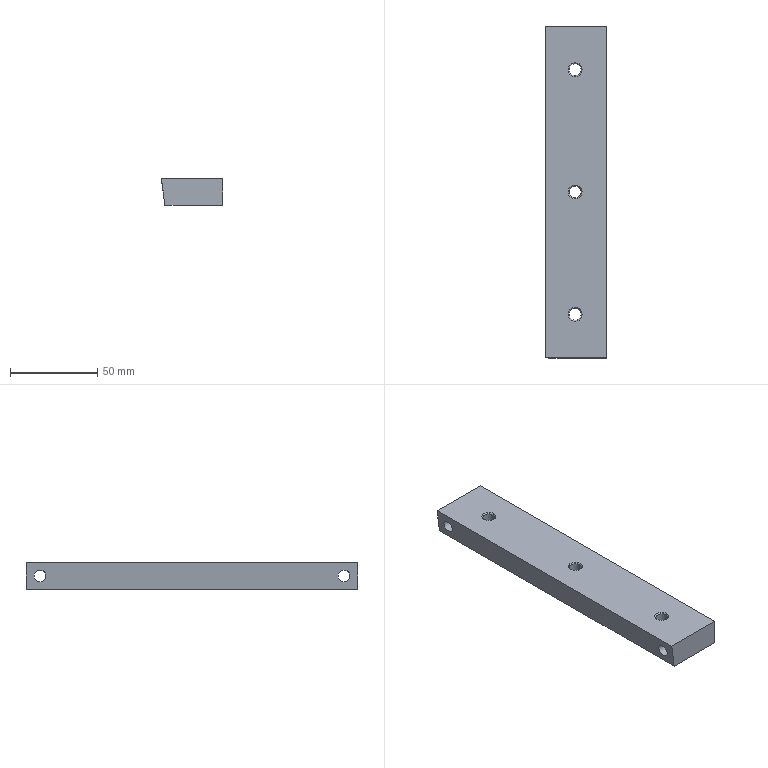Part | STEP file | YBQDJ-QD-5 | 1 solid | 16 faces | box 35 x 190 x 15 mm | volume 92776 mm3 | plane 6 | cylinder 5 | cone 5 | commonest cylinder face diameters 6.8 x5
STEP:
#1=CARTESIAN_POINT('',(0.,0.,0.));
#2=DIRECTION('',(0.,0.,1.));
#3=DIRECTION('',(1.,0.,0.));
#4=AXIS2_PLACEMENT_3D('',#1,#2,#3);
#5=CARTESIAN_POINT('',(-350.,-265.,135.));
#6=VERTEX_POINT('',#5);
#7=CARTESIAN_POINT('',(-354.,-265.,135.));
#8=DIRECTION('',(0.,0.,-1.));
#9=DIRECTION('',(1.,0.,0.));
#10=AXIS2_PLACEMENT_3D('',#7,#8,#9);
#11=CIRCLE('',#10,4.);
#12=CARTESIAN_POINT('',(-341.,1779.,135.));
#13=DIRECTION('',(0.,0.,1.));
#14=DIRECTION('',(1.,0.,0.));
#15=AXIS2_PLACEMENT_3D('',#12,#13,#14);
#16=PLANE('',#15);
#17=CARTESIAN_POINT('',(-9.,-2044.));
#18=CARTESIAN_POINT('',(-9.,-2050.928));
#19=CARTESIAN_POINT('',(-15.,-2047.464));
#20=CARTESIAN_POINT('',(-21.,-2044.));
#21=CARTESIAN_POINT('',(-15.,-2040.536));
#22=CARTESIAN_POINT('',(-9.,-2037.072));
#23=CARTESIAN_POINT('',(-9.,-2044.));
#24=(BOUNDED_CURVE()B_SPLINE_CURVE(2,(#17,#18,#19,#20,#21,#22,#23),.UNSPECIFIED.,.T.,.F.)B_SPLINE_CURVE_WITH_KNOTS((1,2,2,2,2,1),(-2.094,0.,2.094,4.189,6.283,8.378),.UNSPECIFIED.)CURVE()GEOMETRIC_REPRESENTATION_ITEM()RATIONAL_B_SPLINE_CURVE((1.,0.5,1.,0.5,1.,0.5,1.))REPRESENTATION_ITEM(''));
#25=(GEOMETRIC_REPRESENTATION_CONTEXT(2)PARAMETRIC_REPRESENTATION_CONTEXT()REPRESENTATION_CONTEXT('',''));
#26=DEFINITIONAL_REPRESENTATION('',(#24),#25);
#27=PCURVE('',#16,#26);
#28=CARTESIAN_POINT('',(-354.,-265.,134.4));
#29=DIRECTION('',(0.,0.,1.));
#30=DIRECTION('',(1.,0.,0.));
#31=AXIS2_PLACEMENT_3D('',#28,#29,#30);
#32=CONICAL_SURFACE('',#31,3.4,0.7854);
#33=CARTESIAN_POINT('',(6.283,0.6));
#34=DIRECTION('',(-1.,0.));
#35=VECTOR('',#34,1.);
#36=LINE('',#33,#35);
#37=(GEOMETRIC_REPRESENTATION_CONTEXT(2)PARAMETRIC_REPRESENTATION_CONTEXT()REPRESENTATION_CONTEXT('',''));
#38=DEFINITIONAL_REPRESENTATION('',(#36),#37);
#39=PCURVE('',#32,#38);
#40=SURFACE_CURVE('',#11,(#27,#39),.PCURVE_S1.);
#41=EDGE_CURVE('',#6,#6,#40,.T.);
#42=ORIENTED_EDGE('',*,*,#41,.T.);
#43=EDGE_LOOP('',(#42));
#44=FACE_BOUND('',#43,.T.);
#45=CARTESIAN_POINT('',(-350.,-195.,135.));
#46=VERTEX_POINT('',#45);
#47=CARTESIAN_POINT('',(-354.,-195.,135.));
#48=DIRECTION('',(0.,0.,-1.));
#49=DIRECTION('',(1.,0.,0.));
#50=AXIS2_PLACEMENT_3D('',#47,#48,#49);
#51=CIRCLE('',#50,4.);
#52=CARTESIAN_POINT('',(-9.,-1974.));
#53=CARTESIAN_POINT('',(-9.,-1980.928));
#54=CARTESIAN_POINT('',(-15.,-1977.464));
#55=CARTESIAN_POINT('',(-21.,-1974.));
#56=CARTESIAN_POINT('',(-15.,-1970.536));
#57=CARTESIAN_POINT('',(-9.,-1967.072));
#58=CARTESIAN_POINT('',(-9.,-1974.));
#59=(BOUNDED_CURVE()B_SPLINE_CURVE(2,(#52,#53,#54,#55,#56,#57,#58),.UNSPECIFIED.,.T.,.F.)B_SPLINE_CURVE_WITH_KNOTS((1,2,2,2,2,1),(-2.094,0.,2.094,4.189,6.283,8.378),.UNSPECIFIED.)CURVE()GEOMETRIC_REPRESENTATION_ITEM()RATIONAL_B_SPLINE_CURVE((1.,0.5,1.,0.5,1.,0.5,1.))REPRESENTATION_ITEM(''));
#60=(GEOMETRIC_REPRESENTATION_CONTEXT(2)PARAMETRIC_REPRESENTATION_CONTEXT()REPRESENTATION_CONTEXT('',''));
#61=DEFINITIONAL_REPRESENTATION('',(#59),#60);
#62=PCURVE('',#16,#61);
#63=CARTESIAN_POINT('',(-354.,-195.,135.));
#64=DIRECTION('',(0.,0.,1.));
#65=DIRECTION('',(1.,0.,0.));
#66=AXIS2_PLACEMENT_3D('',#63,#64,#65);
#67=CONICAL_SURFACE('',#66,4.,0.7854);
#68=CARTESIAN_POINT('',(6.283,0.));
#69=DIRECTION('',(-1.,0.));
#70=VECTOR('',#69,1.);
#71=LINE('',#68,#70);
#72=(GEOMETRIC_REPRESENTATION_CONTEXT(2)PARAMETRIC_REPRESENTATION_CONTEXT()REPRESENTATION_CONTEXT('',''));
#73=DEFINITIONAL_REPRESENTATION('',(#71),#72);
#74=PCURVE('',#67,#73);
#75=SURFACE_CURVE('',#51,(#62,#74),.PCURVE_S1.);
#76=EDGE_CURVE('',#46,#46,#75,.T.);
#77=ORIENTED_EDGE('',*,*,#76,.T.);
#78=EDGE_LOOP('',(#77));
#79=FACE_BOUND('',#78,.T.);
#80=CARTESIAN_POINT('',(-350.,-125.,135.));
#81=VERTEX_POINT('',#80);
#82=CARTESIAN_POINT('',(-354.,-125.,135.));
#83=DIRECTION('',(0.,0.,-1.));
#84=DIRECTION('',(1.,0.,0.));
#85=AXIS2_PLACEMENT_3D('',#82,#83,#84);
#86=CIRCLE('',#85,4.);
#87=CARTESIAN_POINT('',(-9.,-1904.));
#88=CARTESIAN_POINT('',(-9.,-1910.928));
#89=CARTESIAN_POINT('',(-15.,-1907.464));
#90=CARTESIAN_POINT('',(-21.,-1904.));
#91=CARTESIAN_POINT('',(-15.,-1900.536));
#92=CARTESIAN_POINT('',(-9.,-1897.072));
#93=CARTESIAN_POINT('',(-9.,-1904.));
#94=(BOUNDED_CURVE()B_SPLINE_CURVE(2,(#87,#88,#89,#90,#91,#92,#93),.UNSPECIFIED.,.T.,.F.)B_SPLINE_CURVE_WITH_KNOTS((1,2,2,2,2,1),(-2.094,0.,2.094,4.189,6.283,8.378),.UNSPECIFIED.)CURVE()GEOMETRIC_REPRESENTATION_ITEM()RATIONAL_B_SPLINE_CURVE((1.,0.5,1.,0.5,1.,0.5,1.))REPRESENTATION_ITEM(''));
#95=(GEOMETRIC_REPRESENTATION_CONTEXT(2)PARAMETRIC_REPRESENTATION_CONTEXT()REPRESENTATION_CONTEXT('',''));
#96=DEFINITIONAL_REPRESENTATION('',(#94),#95);
#97=PCURVE('',#16,#96);
#98=CARTESIAN_POINT('',(-354.,-125.,135.));
#99=DIRECTION('',(0.,0.,1.));
#100=DIRECTION('',(1.,0.,0.));
#101=AXIS2_PLACEMENT_3D('',#98,#99,#100);
#102=CONICAL_SURFACE('',#101,4.,0.7854);
#103=CARTESIAN_POINT('',(6.283,0.));
#104=DIRECTION('',(-1.,0.));
#105=VECTOR('',#104,1.);
#106=LINE('',#103,#105);
#107=(GEOMETRIC_REPRESENTATION_CONTEXT(2)PARAMETRIC_REPRESENTATION_CONTEXT()REPRESENTATION_CONTEXT('',''));
#108=DEFINITIONAL_REPRESENTATION('',(#106),#107);
#109=PCURVE('',#102,#108);
#110=SURFACE_CURVE('',#86,(#97,#109),.PCURVE_S1.);
#111=EDGE_CURVE('',#81,#81,#110,.T.);
#112=ORIENTED_EDGE('',*,*,#111,.T.);
#113=EDGE_LOOP('',(#112));
#114=FACE_BOUND('',#113,.T.);
#115=CARTESIAN_POINT('',(-371.,-100.,135.));
#116=VERTEX_POINT('',#115);
#117=CARTESIAN_POINT('',(-336.,-100.,135.));
#118=VERTEX_POINT('',#117);
#119=CARTESIAN_POINT('',(-341.,-100.,135.));
#120=DIRECTION('',(1.,0.,0.));
#121=VECTOR('',#120,1.);
#122=LINE('',#119,#121);
#123=CARTESIAN_POINT('',(0.,-1879.));
#124=DIRECTION('',(1.,0.));
#125=VECTOR('',#124,1.);
#126=LINE('',#123,#125);
#127=(GEOMETRIC_REPRESENTATION_CONTEXT(2)PARAMETRIC_REPRESENTATION_CONTEXT()REPRESENTATION_CONTEXT('',''));
#128=DEFINITIONAL_REPRESENTATION('',(#126),#127);
#129=PCURVE('',#16,#128);
#130=CARTESIAN_POINT('',(-291.5,-100.,264.));
#131=DIRECTION('',(0.,-1.,0.));
#132=DIRECTION('',(0.,0.,1.));
#133=AXIS2_PLACEMENT_3D('',#130,#131,#132);
#134=PLANE('',#133);
#135=CARTESIAN_POINT('',(-129.,49.5));
#136=DIRECTION('',(0.,-1.));
#137=VECTOR('',#136,1.);
#138=LINE('',#135,#137);
#139=(GEOMETRIC_REPRESENTATION_CONTEXT(2)PARAMETRIC_REPRESENTATION_CONTEXT()REPRESENTATION_CONTEXT('',''));
#140=DEFINITIONAL_REPRESENTATION('',(#138),#139);
#141=PCURVE('',#134,#140);
#142=SURFACE_CURVE('',#122,(#129,#141),.PCURVE_S1.);
#143=EDGE_CURVE('',#116,#118,#142,.T.);
#144=ORIENTED_EDGE('',*,*,#143,.F.);
#145=CARTESIAN_POINT('',(-371.,-290.,135.));
#146=VERTEX_POINT('',#145);
#147=CARTESIAN_POINT('',(-371.,1779.,135.));
#148=DIRECTION('',(0.,-1.,0.));
#149=VECTOR('',#148,1.);
#150=LINE('',#147,#149);
#151=CARTESIAN_POINT('',(-30.,0.));
#152=DIRECTION('',(0.,-1.));
#153=VECTOR('',#152,1.);
#154=LINE('',#151,#153);
#155=(GEOMETRIC_REPRESENTATION_CONTEXT(2)PARAMETRIC_REPRESENTATION_CONTEXT()REPRESENTATION_CONTEXT('',''));
#156=DEFINITIONAL_REPRESENTATION('',(#154),#155);
#157=PCURVE('',#16,#156);
#158=CARTESIAN_POINT('',(-371.,-290.,135.));
#159=DIRECTION('',(-0.9912,0.,-0.1322));
#160=DIRECTION('',(-0.1322,0.,0.9912));
#161=AXIS2_PLACEMENT_3D('',#158,#159,#160);
#162=PLANE('',#161);
#163=CARTESIAN_POINT('',(0.,2069.));
#164=DIRECTION('',(0.,-1.));
#165=VECTOR('',#164,1.);
#166=LINE('',#163,#165);
#167=(GEOMETRIC_REPRESENTATION_CONTEXT(2)PARAMETRIC_REPRESENTATION_CONTEXT()REPRESENTATION_CONTEXT('',''));
#168=DEFINITIONAL_REPRESENTATION('',(#166),#167);
#169=PCURVE('',#162,#168);
#170=SURFACE_CURVE('',#150,(#157,#169),.PCURVE_S1.);
#171=EDGE_CURVE('',#116,#146,#170,.T.);
#172=ORIENTED_EDGE('',*,*,#171,.T.);
#173=CARTESIAN_POINT('',(-336.,-290.,135.));
#174=VERTEX_POINT('',#173);
#175=CARTESIAN_POINT('',(164.,-290.,135.));
#176=DIRECTION('',(-1.,0.,0.));
#177=VECTOR('',#176,1.);
#178=LINE('',#175,#177);
#179=CARTESIAN_POINT('',(505.,-2069.));
#180=DIRECTION('',(-1.,0.));
#181=VECTOR('',#180,1.);
#182=LINE('',#179,#181);
#183=(GEOMETRIC_REPRESENTATION_CONTEXT(2)PARAMETRIC_REPRESENTATION_CONTEXT()REPRESENTATION_CONTEXT('',''));
#184=DEFINITIONAL_REPRESENTATION('',(#182),#183);
#185=PCURVE('',#16,#184);
#186=CARTESIAN_POINT('',(164.,-290.,9.));
#187=DIRECTION('',(0.,-1.,0.));
#188=DIRECTION('',(0.,0.,-1.));
#189=AXIS2_PLACEMENT_3D('',#186,#187,#188);
#190=PLANE('',#189);
#191=CARTESIAN_POINT('',(-126.,0.));
#192=DIRECTION('',(0.,-1.));
#193=VECTOR('',#192,1.);
#194=LINE('',#191,#193);
#195=(GEOMETRIC_REPRESENTATION_CONTEXT(2)PARAMETRIC_REPRESENTATION_CONTEXT()REPRESENTATION_CONTEXT('',''));
#196=DEFINITIONAL_REPRESENTATION('',(#194),#195);
#197=PCURVE('',#190,#196);
#198=SURFACE_CURVE('',#178,(#185,#197),.PCURVE_S1.);
#199=EDGE_CURVE('',#174,#146,#198,.T.);
#200=ORIENTED_EDGE('',*,*,#199,.F.);
#201=CARTESIAN_POINT('',(-336.,1779.,135.));
#202=DIRECTION('',(0.,-1.,0.));
#203=VECTOR('',#202,1.);
#204=LINE('',#201,#203);
#205=CARTESIAN_POINT('',(5.,0.));
#206=DIRECTION('',(0.,-1.));
#207=VECTOR('',#206,1.);
#208=LINE('',#205,#207);
#209=(GEOMETRIC_REPRESENTATION_CONTEXT(2)PARAMETRIC_REPRESENTATION_CONTEXT()REPRESENTATION_CONTEXT('',''));
#210=DEFINITIONAL_REPRESENTATION('',(#208),#209);
#211=PCURVE('',#16,#210);
#212=CARTESIAN_POINT('',(-336.,1779.,119.));
#213=DIRECTION('',(1.,0.,0.));
#214=DIRECTION('',(0.,0.,-1.));
#215=AXIS2_PLACEMENT_3D('',#212,#213,#214);
#216=PLANE('',#215);
#217=CARTESIAN_POINT('',(-16.,0.));
#218=DIRECTION('',(0.,-1.));
#219=VECTOR('',#218,1.);
#220=LINE('',#217,#219);
#221=(GEOMETRIC_REPRESENTATION_CONTEXT(2)PARAMETRIC_REPRESENTATION_CONTEXT()REPRESENTATION_CONTEXT('',''));
#222=DEFINITIONAL_REPRESENTATION('',(#220),#221);
#223=PCURVE('',#216,#222);
#224=SURFACE_CURVE('',#204,(#211,#223),.PCURVE_S1.);
#225=EDGE_CURVE('',#118,#174,#224,.T.);
#226=ORIENTED_EDGE('',*,*,#225,.F.);
#227=EDGE_LOOP('',(#144,#172,#200,#226));
#228=FACE_BOUND('',#227,.T.);
#229=ADVANCED_FACE('',(#44,#79,#114,#228),#16,.T.);
#230=CARTESIAN_POINT('',(-357.4,-125.,120.));
#231=VERTEX_POINT('',#230);
#232=CARTESIAN_POINT('',(-350.6,-125.,120.));
#233=VERTEX_POINT('',#232);
#234=CARTESIAN_POINT('',(-354.,-125.,120.));
#235=DIRECTION('',(0.,0.,1.));
#236=DIRECTION('',(-1.,0.,0.));
#237=AXIS2_PLACEMENT_3D('',#234,#235,#236);
#238=CIRCLE('',#237,3.4);
#239=CARTESIAN_POINT('',(-371.,1779.,120.));
#240=DIRECTION('',(0.,0.,-1.));
#241=DIRECTION('',(-1.,0.,0.));
#242=AXIS2_PLACEMENT_3D('',#239,#240,#241);
#243=PLANE('',#242);
#244=CARTESIAN_POINT('',(-13.6,-1904.));
#245=CARTESIAN_POINT('',(-13.6,-1909.889));
#246=CARTESIAN_POINT('',(-18.7,-1906.944));
#247=CARTESIAN_POINT('',(-23.8,-1904.));
#248=CARTESIAN_POINT('',(-18.7,-1901.056));
#249=CARTESIAN_POINT('',(-13.6,-1898.111));
#250=CARTESIAN_POINT('',(-13.6,-1904.));
#251=(BOUNDED_CURVE()B_SPLINE_CURVE(2,(#244,#245,#246,#247,#248,#249,#250),.UNSPECIFIED.,.T.,.F.)B_SPLINE_CURVE_WITH_KNOTS((1,2,2,2,2,1),(-2.094,0.,2.094,4.189,6.283,8.378),.UNSPECIFIED.)CURVE()GEOMETRIC_REPRESENTATION_ITEM()RATIONAL_B_SPLINE_CURVE((1.,0.5,1.,0.5,1.,0.5,1.))REPRESENTATION_ITEM(''));
#252=(GEOMETRIC_REPRESENTATION_CONTEXT(2)PARAMETRIC_REPRESENTATION_CONTEXT()REPRESENTATION_CONTEXT('',''));
#253=DEFINITIONAL_REPRESENTATION('',(#251),#252);
#254=PCURVE('',#243,#253);
#255=CARTESIAN_POINT('',(-354.,-125.,87.));
#256=DIRECTION('',(0.,0.,1.));
#257=DIRECTION('',(1.,0.,0.));
#258=AXIS2_PLACEMENT_3D('',#255,#256,#257);
#259=CYLINDRICAL_SURFACE('',#258,3.4);
#260=CARTESIAN_POINT('',(3.142,33.));
#261=DIRECTION('',(1.,0.));
#262=VECTOR('',#261,1.);
#263=LINE('',#260,#262);
#264=(GEOMETRIC_REPRESENTATION_CONTEXT(2)PARAMETRIC_REPRESENTATION_CONTEXT()REPRESENTATION_CONTEXT('',''));
#265=DEFINITIONAL_REPRESENTATION('',(#263),#264);
#266=PCURVE('',#259,#265);
#267=SURFACE_CURVE('',#238,(#254,#266),.PCURVE_S1.);
#268=EDGE_CURVE('',#231,#233,#267,.T.);
#269=ORIENTED_EDGE('',*,*,#268,.T.);
#270=CARTESIAN_POINT('',(-354.,-125.,120.));
#271=DIRECTION('',(0.,0.,1.));
#272=DIRECTION('',(-1.,0.,0.));
#273=AXIS2_PLACEMENT_3D('',#270,#271,#272);
#274=CIRCLE('',#273,3.4);
#275=CARTESIAN_POINT('',(-13.6,-1904.));
#276=CARTESIAN_POINT('',(-13.6,-1909.889));
#277=CARTESIAN_POINT('',(-18.7,-1906.944));
#278=CARTESIAN_POINT('',(-23.8,-1904.));
#279=CARTESIAN_POINT('',(-18.7,-1901.056));
#280=CARTESIAN_POINT('',(-13.6,-1898.111));
#281=CARTESIAN_POINT('',(-13.6,-1904.));
#282=(BOUNDED_CURVE()B_SPLINE_CURVE(2,(#275,#276,#277,#278,#279,#280,#281),.UNSPECIFIED.,.T.,.F.)B_SPLINE_CURVE_WITH_KNOTS((1,2,2,2,2,1),(-2.094,0.,2.094,4.189,6.283,8.378),.UNSPECIFIED.)CURVE()GEOMETRIC_REPRESENTATION_ITEM()RATIONAL_B_SPLINE_CURVE((1.,0.5,1.,0.5,1.,0.5,1.))REPRESENTATION_ITEM(''));
#283=(GEOMETRIC_REPRESENTATION_CONTEXT(2)PARAMETRIC_REPRESENTATION_CONTEXT()REPRESENTATION_CONTEXT('',''));
#284=DEFINITIONAL_REPRESENTATION('',(#282),#283);
#285=PCURVE('',#243,#284);
#286=CARTESIAN_POINT('',(-3.142,33.));
#287=DIRECTION('',(1.,0.));
#288=VECTOR('',#287,1.);
#289=LINE('',#286,#288);
#290=(GEOMETRIC_REPRESENTATION_CONTEXT(2)PARAMETRIC_REPRESENTATION_CONTEXT()REPRESENTATION_CONTEXT('',''));
#291=DEFINITIONAL_REPRESENTATION('',(#289),#290);
#292=PCURVE('',#259,#291);
#293=SURFACE_CURVE('',#274,(#285,#292),.PCURVE_S1.);
#294=EDGE_CURVE('',#233,#231,#293,.T.);
#295=ORIENTED_EDGE('',*,*,#294,.T.);
#296=EDGE_LOOP('',(#269,#295));
#297=FACE_BOUND('',#296,.T.);
#298=CARTESIAN_POINT('',(-357.4,-195.,120.));
#299=VERTEX_POINT('',#298);
#300=CARTESIAN_POINT('',(-350.6,-195.,120.));
#301=VERTEX_POINT('',#300);
#302=CARTESIAN_POINT('',(-354.,-195.,120.));
#303=DIRECTION('',(0.,0.,1.));
#304=DIRECTION('',(-1.,0.,0.));
#305=AXIS2_PLACEMENT_3D('',#302,#303,#304);
#306=CIRCLE('',#305,3.4);
#307=CARTESIAN_POINT('',(-13.6,-1974.));
#308=CARTESIAN_POINT('',(-13.6,-1979.889));
#309=CARTESIAN_POINT('',(-18.7,-1976.944));
#310=CARTESIAN_POINT('',(-23.8,-1974.));
#311=CARTESIAN_POINT('',(-18.7,-1971.056));
#312=CARTESIAN_POINT('',(-13.6,-1968.111));
#313=CARTESIAN_POINT('',(-13.6,-1974.));
#314=(BOUNDED_CURVE()B_SPLINE_CURVE(2,(#307,#308,#309,#310,#311,#312,#313),.UNSPECIFIED.,.T.,.F.)B_SPLINE_CURVE_WITH_KNOTS((1,2,2,2,2,1),(-2.094,0.,2.094,4.189,6.283,8.378),.UNSPECIFIED.)CURVE()GEOMETRIC_REPRESENTATION_ITEM()RATIONAL_B_SPLINE_CURVE((1.,0.5,1.,0.5,1.,0.5,1.))REPRESENTATION_ITEM(''));
#315=(GEOMETRIC_REPRESENTATION_CONTEXT(2)PARAMETRIC_REPRESENTATION_CONTEXT()REPRESENTATION_CONTEXT('',''));
#316=DEFINITIONAL_REPRESENTATION('',(#314),#315);
#317=PCURVE('',#243,#316);
#318=CARTESIAN_POINT('',(-354.,-195.,87.));
#319=DIRECTION('',(0.,0.,1.));
#320=DIRECTION('',(1.,0.,0.));
#321=AXIS2_PLACEMENT_3D('',#318,#319,#320);
#322=CYLINDRICAL_SURFACE('',#321,3.4);
#323=CARTESIAN_POINT('',(3.142,33.));
#324=DIRECTION('',(1.,0.));
#325=VECTOR('',#324,1.);
#326=LINE('',#323,#325);
#327=(GEOMETRIC_REPRESENTATION_CONTEXT(2)PARAMETRIC_REPRESENTATION_CONTEXT()REPRESENTATION_CONTEXT('',''));
#328=DEFINITIONAL_REPRESENTATION('',(#326),#327);
#329=PCURVE('',#322,#328);
#330=SURFACE_CURVE('',#306,(#317,#329),.PCURVE_S1.);
#331=EDGE_CURVE('',#299,#301,#330,.T.);
#332=ORIENTED_EDGE('',*,*,#331,.T.);
#333=CARTESIAN_POINT('',(-354.,-195.,120.));
#334=DIRECTION('',(0.,0.,1.));
#335=DIRECTION('',(-1.,0.,0.));
#336=AXIS2_PLACEMENT_3D('',#333,#334,#335);
#337=CIRCLE('',#336,3.4);
#338=CARTESIAN_POINT('',(-13.6,-1974.));
#339=CARTESIAN_POINT('',(-13.6,-1979.889));
#340=CARTESIAN_POINT('',(-18.7,-1976.944));
#341=CARTESIAN_POINT('',(-23.8,-1974.));
#342=CARTESIAN_POINT('',(-18.7,-1971.056));
#343=CARTESIAN_POINT('',(-13.6,-1968.111));
#344=CARTESIAN_POINT('',(-13.6,-1974.));
#345=(BOUNDED_CURVE()B_SPLINE_CURVE(2,(#338,#339,#340,#341,#342,#343,#344),.UNSPECIFIED.,.T.,.F.)B_SPLINE_CURVE_WITH_KNOTS((1,2,2,2,2,1),(-2.094,0.,2.094,4.189,6.283,8.378),.UNSPECIFIED.)CURVE()GEOMETRIC_REPRESENTATION_ITEM()RATIONAL_B_SPLINE_CURVE((1.,0.5,1.,0.5,1.,0.5,1.))REPRESENTATION_ITEM(''));
#346=(GEOMETRIC_REPRESENTATION_CONTEXT(2)PARAMETRIC_REPRESENTATION_CONTEXT()REPRESENTATION_CONTEXT('',''));
#347=DEFINITIONAL_REPRESENTATION('',(#345),#346);
#348=PCURVE('',#243,#347);
#349=CARTESIAN_POINT('',(-3.142,33.));
#350=DIRECTION('',(1.,0.));
#351=VECTOR('',#350,1.);
#352=LINE('',#349,#351);
#353=(GEOMETRIC_REPRESENTATION_CONTEXT(2)PARAMETRIC_REPRESENTATION_CONTEXT()REPRESENTATION_CONTEXT('',''));
#354=DEFINITIONAL_REPRESENTATION('',(#352),#353);
#355=PCURVE('',#322,#354);
#356=SURFACE_CURVE('',#337,(#348,#355),.PCURVE_S1.);
#357=EDGE_CURVE('',#301,#299,#356,.T.);
#358=ORIENTED_EDGE('',*,*,#357,.T.);
#359=EDGE_LOOP('',(#332,#358));
#360=FACE_BOUND('',#359,.T.);
#361=CARTESIAN_POINT('',(-369.,-290.,120.));
#362=VERTEX_POINT('',#361);
#363=CARTESIAN_POINT('',(-336.,-290.,120.));
#364=VERTEX_POINT('',#363);
#365=CARTESIAN_POINT('',(164.,-290.,120.));
#366=DIRECTION('',(1.,0.,0.));
#367=VECTOR('',#366,1.);
#368=LINE('',#365,#367);
#369=CARTESIAN_POINT('',(-535.,-2069.));
#370=DIRECTION('',(-1.,0.));
#371=VECTOR('',#370,1.);
#372=LINE('',#369,#371);
#373=(GEOMETRIC_REPRESENTATION_CONTEXT(2)PARAMETRIC_REPRESENTATION_CONTEXT()REPRESENTATION_CONTEXT('',''));
#374=DEFINITIONAL_REPRESENTATION('',(#372),#373);
#375=PCURVE('',#243,#374);
#376=CARTESIAN_POINT('',(-111.,0.));
#377=DIRECTION('',(0.,1.));
#378=VECTOR('',#377,1.);
#379=LINE('',#376,#378);
#380=(GEOMETRIC_REPRESENTATION_CONTEXT(2)PARAMETRIC_REPRESENTATION_CONTEXT()REPRESENTATION_CONTEXT('',''));
#381=DEFINITIONAL_REPRESENTATION('',(#379),#380);
#382=PCURVE('',#190,#381);
#383=SURFACE_CURVE('',#368,(#375,#382),.PCURVE_S1.);
#384=EDGE_CURVE('',#362,#364,#383,.T.);
#385=ORIENTED_EDGE('',*,*,#384,.F.);
#386=CARTESIAN_POINT('',(-369.,-100.,120.));
#387=VERTEX_POINT('',#386);
#388=CARTESIAN_POINT('',(-369.,1779.,120.));
#389=DIRECTION('',(0.,1.,0.));
#390=VECTOR('',#389,1.);
#391=LINE('',#388,#390);
#392=CARTESIAN_POINT('',(-2.,0.));
#393=DIRECTION('',(0.,1.));
#394=VECTOR('',#393,1.);
#395=LINE('',#392,#394);
#396=(GEOMETRIC_REPRESENTATION_CONTEXT(2)PARAMETRIC_REPRESENTATION_CONTEXT()REPRESENTATION_CONTEXT('',''));
#397=DEFINITIONAL_REPRESENTATION('',(#395),#396);
#398=PCURVE('',#243,#397);
#399=CARTESIAN_POINT('',(-15.133,2069.));
#400=DIRECTION('',(0.,1.));
#401=VECTOR('',#400,1.);
#402=LINE('',#399,#401);
#403=(GEOMETRIC_REPRESENTATION_CONTEXT(2)PARAMETRIC_REPRESENTATION_CONTEXT()REPRESENTATION_CONTEXT('',''));
#404=DEFINITIONAL_REPRESENTATION('',(#402),#403);
#405=PCURVE('',#162,#404);
#406=SURFACE_CURVE('',#391,(#398,#405),.PCURVE_S1.);
#407=EDGE_CURVE('',#362,#387,#406,.T.);
#408=ORIENTED_EDGE('',*,*,#407,.T.);
#409=CARTESIAN_POINT('',(-336.,-100.,120.));
#410=VERTEX_POINT('',#409);
#411=CARTESIAN_POINT('',(-371.,-100.,120.));
#412=DIRECTION('',(-1.,0.,0.));
#413=VECTOR('',#412,1.);
#414=LINE('',#411,#413);
#415=CARTESIAN_POINT('',(0.,-1879.));
#416=DIRECTION('',(1.,0.));
#417=VECTOR('',#416,1.);
#418=LINE('',#415,#417);
#419=(GEOMETRIC_REPRESENTATION_CONTEXT(2)PARAMETRIC_REPRESENTATION_CONTEXT()REPRESENTATION_CONTEXT('',''));
#420=DEFINITIONAL_REPRESENTATION('',(#418),#419);
#421=PCURVE('',#243,#420);
#422=CARTESIAN_POINT('',(-144.,79.5));
#423=DIRECTION('',(0.,1.));
#424=VECTOR('',#423,1.);
#425=LINE('',#422,#424);
#426=(GEOMETRIC_REPRESENTATION_CONTEXT(2)PARAMETRIC_REPRESENTATION_CONTEXT()REPRESENTATION_CONTEXT('',''));
#427=DEFINITIONAL_REPRESENTATION('',(#425),#426);
#428=PCURVE('',#134,#427);
#429=SURFACE_CURVE('',#414,(#421,#428),.PCURVE_S1.);
#430=EDGE_CURVE('',#410,#387,#429,.T.);
#431=ORIENTED_EDGE('',*,*,#430,.F.);
#432=CARTESIAN_POINT('',(-336.,1779.,120.));
#433=DIRECTION('',(0.,-1.,0.));
#434=VECTOR('',#433,1.);
#435=LINE('',#432,#434);
#436=CARTESIAN_POINT('',(-35.,0.));
#437=DIRECTION('',(0.,-1.));
#438=VECTOR('',#437,1.);
#439=LINE('',#436,#438);
#440=(GEOMETRIC_REPRESENTATION_CONTEXT(2)PARAMETRIC_REPRESENTATION_CONTEXT()REPRESENTATION_CONTEXT('',''));
#441=DEFINITIONAL_REPRESENTATION('',(#439),#440);
#442=PCURVE('',#243,#441);
#443=CARTESIAN_POINT('',(-1.,0.));
#444=DIRECTION('',(0.,-1.));
#445=VECTOR('',#444,1.);
#446=LINE('',#443,#445);
#447=(GEOMETRIC_REPRESENTATION_CONTEXT(2)PARAMETRIC_REPRESENTATION_CONTEXT()REPRESENTATION_CONTEXT('',''));
#448=DEFINITIONAL_REPRESENTATION('',(#446),#447);
#449=PCURVE('',#216,#448);
#450=SURFACE_CURVE('',#435,(#442,#449),.PCURVE_S1.);
#451=EDGE_CURVE('',#410,#364,#450,.T.);
#452=ORIENTED_EDGE('',*,*,#451,.T.);
#453=EDGE_LOOP('',(#385,#408,#431,#452));
#454=FACE_BOUND('',#453,.T.);
#455=CARTESIAN_POINT('',(-357.4,-265.,120.));
#456=VERTEX_POINT('',#455);
#457=CARTESIAN_POINT('',(-350.6,-265.,120.));
#458=VERTEX_POINT('',#457);
#459=CARTESIAN_POINT('',(-354.,-265.,120.));
#460=DIRECTION('',(0.,0.,-1.));
#461=DIRECTION('',(-1.,0.,0.));
#462=AXIS2_PLACEMENT_3D('',#459,#460,#461);
#463=CIRCLE('',#462,3.4);
#464=CARTESIAN_POINT('',(-17.,-2044.));
#465=DIRECTION('',(1.,0.));
#466=AXIS2_PLACEMENT_2D('',#464,#465);
#467=CIRCLE('',#466,3.4);
#468=(GEOMETRIC_REPRESENTATION_CONTEXT(2)PARAMETRIC_REPRESENTATION_CONTEXT()REPRESENTATION_CONTEXT('',''));
#469=DEFINITIONAL_REPRESENTATION('',(#467),#468);
#470=PCURVE('',#243,#469);
#471=CARTESIAN_POINT('',(-354.,-265.,87.));
#472=DIRECTION('',(0.,0.,1.));
#473=DIRECTION('',(1.,0.,0.));
#474=AXIS2_PLACEMENT_3D('',#471,#472,#473);
#475=CYLINDRICAL_SURFACE('',#474,3.4);
#476=CARTESIAN_POINT('',(3.142,33.));
#477=DIRECTION('',(-1.,0.));
#478=VECTOR('',#477,1.);
#479=LINE('',#476,#478);
#480=(GEOMETRIC_REPRESENTATION_CONTEXT(2)PARAMETRIC_REPRESENTATION_CONTEXT()REPRESENTATION_CONTEXT('',''));
#481=DEFINITIONAL_REPRESENTATION('',(#479),#480);
#482=PCURVE('',#475,#481);
#483=SURFACE_CURVE('',#463,(#470,#482),.PCURVE_S1.);
#484=EDGE_CURVE('',#456,#458,#483,.T.);
#485=ORIENTED_EDGE('',*,*,#484,.F.);
#486=CARTESIAN_POINT('',(-354.,-265.,120.));
#487=DIRECTION('',(0.,0.,-1.));
#488=DIRECTION('',(-1.,0.,0.));
#489=AXIS2_PLACEMENT_3D('',#486,#487,#488);
#490=CIRCLE('',#489,3.4);
#491=CARTESIAN_POINT('',(-17.,-2044.));
#492=DIRECTION('',(1.,0.));
#493=AXIS2_PLACEMENT_2D('',#491,#492);
#494=CIRCLE('',#493,3.4);
#495=(GEOMETRIC_REPRESENTATION_CONTEXT(2)PARAMETRIC_REPRESENTATION_CONTEXT()REPRESENTATION_CONTEXT('',''));
#496=DEFINITIONAL_REPRESENTATION('',(#494),#495);
#497=PCURVE('',#243,#496);
#498=CARTESIAN_POINT('',(9.425,33.));
#499=DIRECTION('',(-1.,0.));
#500=VECTOR('',#499,1.);
#501=LINE('',#498,#500);
#502=(GEOMETRIC_REPRESENTATION_CONTEXT(2)PARAMETRIC_REPRESENTATION_CONTEXT()REPRESENTATION_CONTEXT('',''));
#503=DEFINITIONAL_REPRESENTATION('',(#501),#502);
#504=PCURVE('',#475,#503);
#505=SURFACE_CURVE('',#490,(#497,#504),.PCURVE_S1.);
#506=EDGE_CURVE('',#458,#456,#505,.T.);
#507=ORIENTED_EDGE('',*,*,#506,.F.);
#508=EDGE_LOOP('',(#485,#507));
#509=FACE_BOUND('',#508,.T.);
#510=ADVANCED_FACE('',(#297,#360,#454,#509),#243,.T.);
#511=CARTESIAN_POINT('',(-336.,-282.,123.5));
#512=VERTEX_POINT('',#511);
#513=CARTESIAN_POINT('',(-336.,-282.,127.5));
#514=DIRECTION('',(-1.,0.,0.));
#515=DIRECTION('',(0.,0.,-1.));
#516=AXIS2_PLACEMENT_3D('',#513,#514,#515);
#517=CIRCLE('',#516,4.);
#518=CARTESIAN_POINT('',(-4.5,-2061.));
#519=CARTESIAN_POINT('',(-4.5,-2067.928));
#520=CARTESIAN_POINT('',(-10.5,-2064.464));
#521=CARTESIAN_POINT('',(-16.5,-2061.));
#522=CARTESIAN_POINT('',(-10.5,-2057.536));
#523=CARTESIAN_POINT('',(-4.5,-2054.072));
#524=CARTESIAN_POINT('',(-4.5,-2061.));
#525=(BOUNDED_CURVE()B_SPLINE_CURVE(2,(#518,#519,#520,#521,#522,#523,#524),.UNSPECIFIED.,.T.,.F.)B_SPLINE_CURVE_WITH_KNOTS((1,2,2,2,2,1),(-2.094,0.,2.094,4.189,6.283,8.378),.UNSPECIFIED.)CURVE()GEOMETRIC_REPRESENTATION_ITEM()RATIONAL_B_SPLINE_CURVE((1.,0.5,1.,0.5,1.,0.5,1.))REPRESENTATION_ITEM(''));
#526=(GEOMETRIC_REPRESENTATION_CONTEXT(2)PARAMETRIC_REPRESENTATION_CONTEXT()REPRESENTATION_CONTEXT('',''));
#527=DEFINITIONAL_REPRESENTATION('',(#525),#526);
#528=PCURVE('',#216,#527);
#529=CARTESIAN_POINT('',(-336.,-282.,127.5));
#530=DIRECTION('',(1.,0.,0.));
#531=DIRECTION('',(0.,0.,-1.));
#532=AXIS2_PLACEMENT_3D('',#529,#530,#531);
#533=CONICAL_SURFACE('',#532,4.,0.7854);
#534=CARTESIAN_POINT('',(6.283,0.));
#535=DIRECTION('',(-1.,0.));
#536=VECTOR('',#535,1.);
#537=LINE('',#534,#536);
#538=(GEOMETRIC_REPRESENTATION_CONTEXT(2)PARAMETRIC_REPRESENTATION_CONTEXT()REPRESENTATION_CONTEXT('',''));
#539=DEFINITIONAL_REPRESENTATION('',(#537),#538);
#540=PCURVE('',#533,#539);
#541=SURFACE_CURVE('',#517,(#528,#540),.PCURVE_S1.);
#542=EDGE_CURVE('',#512,#512,#541,.T.);
#543=ORIENTED_EDGE('',*,*,#542,.T.);
#544=EDGE_LOOP('',(#543));
#545=FACE_BOUND('',#544,.T.);
#546=CARTESIAN_POINT('',(-336.,-108.,123.5));
#547=VERTEX_POINT('',#546);
#548=CARTESIAN_POINT('',(-336.,-108.,127.5));
#549=DIRECTION('',(-1.,0.,0.));
#550=DIRECTION('',(0.,0.,-1.));
#551=AXIS2_PLACEMENT_3D('',#548,#549,#550);
#552=CIRCLE('',#551,4.);
#553=CARTESIAN_POINT('',(-4.5,-1887.));
#554=CARTESIAN_POINT('',(-4.5,-1893.928));
#555=CARTESIAN_POINT('',(-10.5,-1890.464));
#556=CARTESIAN_POINT('',(-16.5,-1887.));
#557=CARTESIAN_POINT('',(-10.5,-1883.536));
#558=CARTESIAN_POINT('',(-4.5,-1880.072));
#559=CARTESIAN_POINT('',(-4.5,-1887.));
#560=(BOUNDED_CURVE()B_SPLINE_CURVE(2,(#553,#554,#555,#556,#557,#558,#559),.UNSPECIFIED.,.T.,.F.)B_SPLINE_CURVE_WITH_KNOTS((1,2,2,2,2,1),(-2.094,0.,2.094,4.189,6.283,8.378),.UNSPECIFIED.)CURVE()GEOMETRIC_REPRESENTATION_ITEM()RATIONAL_B_SPLINE_CURVE((1.,0.5,1.,0.5,1.,0.5,1.))REPRESENTATION_ITEM(''));
#561=(GEOMETRIC_REPRESENTATION_CONTEXT(2)PARAMETRIC_REPRESENTATION_CONTEXT()REPRESENTATION_CONTEXT('',''));
#562=DEFINITIONAL_REPRESENTATION('',(#560),#561);
#563=PCURVE('',#216,#562);
#564=CARTESIAN_POINT('',(-336.,-108.,127.5));
#565=DIRECTION('',(1.,0.,0.));
#566=DIRECTION('',(0.,0.,-1.));
#567=AXIS2_PLACEMENT_3D('',#564,#565,#566);
#568=CONICAL_SURFACE('',#567,4.,0.7854);
#569=CARTESIAN_POINT('',(6.283,0.));
#570=DIRECTION('',(-1.,0.));
#571=VECTOR('',#570,1.);
#572=LINE('',#569,#571);
#573=(GEOMETRIC_REPRESENTATION_CONTEXT(2)PARAMETRIC_REPRESENTATION_CONTEXT()REPRESENTATION_CONTEXT('',''));
#574=DEFINITIONAL_REPRESENTATION('',(#572),#573);
#575=PCURVE('',#568,#574);
#576=SURFACE_CURVE('',#552,(#563,#575),.PCURVE_S1.);
#577=EDGE_CURVE('',#547,#547,#576,.T.);
#578=ORIENTED_EDGE('',*,*,#577,.T.);
#579=EDGE_LOOP('',(#578));
#580=FACE_BOUND('',#579,.T.);
#581=CARTESIAN_POINT('',(-336.,-100.,119.));
#582=DIRECTION('',(0.,0.,-1.));
#583=VECTOR('',#582,1.);
#584=LINE('',#581,#583);
#585=CARTESIAN_POINT('',(0.,-1879.));
#586=DIRECTION('',(1.,0.));
#587=VECTOR('',#586,1.);
#588=LINE('',#585,#587);
#589=(GEOMETRIC_REPRESENTATION_CONTEXT(2)PARAMETRIC_REPRESENTATION_CONTEXT()REPRESENTATION_CONTEXT('',''));
#590=DEFINITIONAL_REPRESENTATION('',(#588),#589);
#591=PCURVE('',#216,#590);
#592=CARTESIAN_POINT('',(-145.,44.5));
#593=DIRECTION('',(-1.,0.));
#594=VECTOR('',#593,1.);
#595=LINE('',#592,#594);
#596=(GEOMETRIC_REPRESENTATION_CONTEXT(2)PARAMETRIC_REPRESENTATION_CONTEXT()REPRESENTATION_CONTEXT('',''));
#597=DEFINITIONAL_REPRESENTATION('',(#595),#596);
#598=PCURVE('',#134,#597);
#599=SURFACE_CURVE('',#584,(#591,#598),.PCURVE_S1.);
#600=EDGE_CURVE('',#118,#410,#599,.T.);
#601=ORIENTED_EDGE('',*,*,#600,.F.);
#602=ORIENTED_EDGE('',*,*,#225,.T.);
#603=CARTESIAN_POINT('',(-336.,-290.,9.));
#604=DIRECTION('',(0.,0.,1.));
#605=VECTOR('',#604,1.);
#606=LINE('',#603,#605);
#607=CARTESIAN_POINT('',(110.,-2069.));
#608=DIRECTION('',(-1.,0.));
#609=VECTOR('',#608,1.);
#610=LINE('',#607,#609);
#611=(GEOMETRIC_REPRESENTATION_CONTEXT(2)PARAMETRIC_REPRESENTATION_CONTEXT()REPRESENTATION_CONTEXT('',''));
#612=DEFINITIONAL_REPRESENTATION('',(#610),#611);
#613=PCURVE('',#216,#612);
#614=CARTESIAN_POINT('',(0.,-500.));
#615=DIRECTION('',(-1.,0.));
#616=VECTOR('',#615,1.);
#617=LINE('',#614,#616);
#618=(GEOMETRIC_REPRESENTATION_CONTEXT(2)PARAMETRIC_REPRESENTATION_CONTEXT()REPRESENTATION_CONTEXT('',''));
#619=DEFINITIONAL_REPRESENTATION('',(#617),#618);
#620=PCURVE('',#190,#619);
#621=SURFACE_CURVE('',#606,(#613,#620),.PCURVE_S1.);
#622=EDGE_CURVE('',#364,#174,#621,.T.);
#623=ORIENTED_EDGE('',*,*,#622,.F.);
#624=ORIENTED_EDGE('',*,*,#451,.F.);
#625=EDGE_LOOP('',(#601,#602,#623,#624));
#626=FACE_BOUND('',#625,.T.);
#627=ADVANCED_FACE('',(#545,#580,#626),#216,.T.);
#628=CARTESIAN_POINT('',(-345.148,-290.,-58.886));
#629=DIRECTION('',(0.1322,0.,-0.9912));
#630=VECTOR('',#629,1.);
#631=LINE('',#628,#630);
#632=CARTESIAN_POINT('',(67.886,-509.148));
#633=DIRECTION('',(0.9912,0.1322));
#634=VECTOR('',#633,1.);
#635=LINE('',#632,#634);
#636=(GEOMETRIC_REPRESENTATION_CONTEXT(2)PARAMETRIC_REPRESENTATION_CONTEXT()REPRESENTATION_CONTEXT('',''));
#637=DEFINITIONAL_REPRESENTATION('',(#635),#636);
#638=PCURVE('',#190,#637);
#639=CARTESIAN_POINT('',(-195.602,0.));
#640=DIRECTION('',(-1.,0.));
#641=VECTOR('',#640,1.);
#642=LINE('',#639,#641);
#643=(GEOMETRIC_REPRESENTATION_CONTEXT(2)PARAMETRIC_REPRESENTATION_CONTEXT()REPRESENTATION_CONTEXT('',''));
#644=DEFINITIONAL_REPRESENTATION('',(#642),#643);
#645=PCURVE('',#162,#644);
#646=SURFACE_CURVE('',#631,(#638,#645),.PCURVE_S1.);
#647=EDGE_CURVE('',#146,#362,#646,.T.);
#648=ORIENTED_EDGE('',*,*,#647,.T.);
#649=ORIENTED_EDGE('',*,*,#384,.T.);
#650=ORIENTED_EDGE('',*,*,#622,.T.);
#651=ORIENTED_EDGE('',*,*,#199,.T.);
#652=EDGE_LOOP('',(#648,#649,#650,#651));
#653=FACE_BOUND('',#652,.T.);
#654=ADVANCED_FACE('',(#653),#190,.T.);
#655=CARTESIAN_POINT('',(-386.511,-100.,251.332));
#656=DIRECTION('',(0.1322,0.,-0.9912));
#657=VECTOR('',#656,1.);
#658=LINE('',#655,#657);
#659=CARTESIAN_POINT('',(117.361,190.));
#660=DIRECTION('',(-1.,0.));
#661=VECTOR('',#660,1.);
#662=LINE('',#659,#661);
#663=(GEOMETRIC_REPRESENTATION_CONTEXT(2)PARAMETRIC_REPRESENTATION_CONTEXT()REPRESENTATION_CONTEXT('',''));
#664=DEFINITIONAL_REPRESENTATION('',(#662),#663);
#665=PCURVE('',#162,#664);
#666=CARTESIAN_POINT('',(-12.668,95.011));
#667=DIRECTION('',(-0.9912,-0.1322));
#668=VECTOR('',#667,1.);
#669=LINE('',#666,#668);
#670=(GEOMETRIC_REPRESENTATION_CONTEXT(2)PARAMETRIC_REPRESENTATION_CONTEXT()REPRESENTATION_CONTEXT('',''));
#671=DEFINITIONAL_REPRESENTATION('',(#669),#670);
#672=PCURVE('',#134,#671);
#673=SURFACE_CURVE('',#658,(#665,#672),.PCURVE_S1.);
#674=EDGE_CURVE('',#116,#387,#673,.T.);
#675=ORIENTED_EDGE('',*,*,#674,.T.);
#676=ORIENTED_EDGE('',*,*,#407,.F.);
#677=ORIENTED_EDGE('',*,*,#647,.F.);
#678=ORIENTED_EDGE('',*,*,#171,.F.);
#679=EDGE_LOOP('',(#675,#676,#677,#678));
#680=FACE_BOUND('',#679,.T.);
#681=CARTESIAN_POINT('',(-369.547,-282.,124.1));
#682=VERTEX_POINT('',#681);
#683=CARTESIAN_POINT('',(-370.,-282.,127.5));
#684=DIRECTION('',(0.9912,0.,0.1322));
#685=DIRECTION('',(0.1322,0.,-0.9912));
#686=AXIS2_PLACEMENT_3D('',#683,#684,#685);
#687=ELLIPSE('',#686,3.43,3.4);
#688=CARTESIAN_POINT('',(-10.996,8.));
#689=CARTESIAN_POINT('',(-10.996,13.889));
#690=CARTESIAN_POINT('',(-5.851,10.944));
#691=CARTESIAN_POINT('',(-0.7062,8.));
#692=CARTESIAN_POINT('',(-5.851,5.056));
#693=CARTESIAN_POINT('',(-10.996,2.111));
#694=CARTESIAN_POINT('',(-10.996,8.));
#695=(BOUNDED_CURVE()B_SPLINE_CURVE(2,(#688,#689,#690,#691,#692,#693,#694),.UNSPECIFIED.,.T.,.F.)B_SPLINE_CURVE_WITH_KNOTS((1,2,2,2,2,1),(-2.094,0.,2.094,4.189,6.283,8.378),.UNSPECIFIED.)CURVE()GEOMETRIC_REPRESENTATION_ITEM()RATIONAL_B_SPLINE_CURVE((1.,0.5,1.,0.5,1.,0.5,1.))REPRESENTATION_ITEM(''));
#696=(GEOMETRIC_REPRESENTATION_CONTEXT(2)PARAMETRIC_REPRESENTATION_CONTEXT()REPRESENTATION_CONTEXT('',''));
#697=DEFINITIONAL_REPRESENTATION('',(#695),#696);
#698=PCURVE('',#162,#697);
#699=CARTESIAN_POINT('',(-369.5,-282.,127.5));
#700=DIRECTION('',(1.,0.,0.));
#701=DIRECTION('',(0.,0.,-1.));
#702=AXIS2_PLACEMENT_3D('',#699,#700,#701);
#703=CYLINDRICAL_SURFACE('',#702,3.4);
#704=CARTESIAN_POINT('',(0.,-0.04667));
#705=CARTESIAN_POINT('',(0.0952,-0.04643));
#706=CARTESIAN_POINT('',(0.2856,-0.05919));
#707=CARTESIAN_POINT('',(0.5712,-0.1134));
#708=CARTESIAN_POINT('',(0.8568,-0.1991));
#709=CARTESIAN_POINT('',(1.142,-0.3091));
#710=CARTESIAN_POINT('',(1.428,-0.4346));
#711=CARTESIAN_POINT('',(1.714,-0.5654));
#712=CARTESIAN_POINT('',(1.999,-0.6909));
#713=CARTESIAN_POINT('',(2.285,-0.8009));
#714=CARTESIAN_POINT('',(2.57,-0.8866));
#715=CARTESIAN_POINT('',(2.856,-0.9409));
#716=CARTESIAN_POINT('',(3.142,-0.9595));
#717=CARTESIAN_POINT('',(3.427,-0.9409));
#718=CARTESIAN_POINT('',(3.713,-0.8866));
#719=CARTESIAN_POINT('',(3.998,-0.8009));
#720=CARTESIAN_POINT('',(4.284,-0.6909));
#721=CARTESIAN_POINT('',(4.57,-0.5654));
#722=CARTESIAN_POINT('',(4.855,-0.4346));
#723=CARTESIAN_POINT('',(5.141,-0.3091));
#724=CARTESIAN_POINT('',(5.426,-0.1991));
#725=CARTESIAN_POINT('',(5.712,-0.1134));
#726=CARTESIAN_POINT('',(5.998,-0.05919));
#727=CARTESIAN_POINT('',(6.188,-0.04643));
#728=CARTESIAN_POINT('',(6.283,-0.04667));
#729=B_SPLINE_CURVE_WITH_KNOTS('',3,(#704,#705,#706,#707,#708,#709,#710,#711,#712,#713,#714,#715,#716,#717,#718,#719,#720,#721,#722,#723,#724,#725,#726,#727,#728),.UNSPECIFIED.,.F.,.F.,(4,1,1,1,1,1,1,1,1,1,1,1,1,1,1,1,1,1,1,1,1,1,4),(0.,0.2856,0.5712,0.8568,1.142,1.428,1.714,1.999,2.285,2.57,2.856,3.142,3.427,3.713,3.998,4.284,4.57,4.855,5.141,5.426,5.712,5.998,6.283),.QUASI_UNIFORM_KNOTS.);
#730=(GEOMETRIC_REPRESENTATION_CONTEXT(2)PARAMETRIC_REPRESENTATION_CONTEXT()REPRESENTATION_CONTEXT('',''));
#731=DEFINITIONAL_REPRESENTATION('',(#729),#730);
#732=PCURVE('',#703,#731);
#733=SURFACE_CURVE('',#687,(#698,#732),.PCURVE_S1.);
#734=EDGE_CURVE('',#682,#682,#733,.T.);
#735=ORIENTED_EDGE('',*,*,#734,.T.);
#736=EDGE_LOOP('',(#735));
#737=FACE_BOUND('',#736,.T.);
#738=CARTESIAN_POINT('',(-369.547,-108.,124.1));
#739=VERTEX_POINT('',#738);
#740=CARTESIAN_POINT('',(-370.,-108.,127.5));
#741=DIRECTION('',(0.9912,0.,0.1322));
#742=DIRECTION('',(0.1322,0.,-0.9912));
#743=AXIS2_PLACEMENT_3D('',#740,#741,#742);
#744=ELLIPSE('',#743,3.43,3.4);
#745=CARTESIAN_POINT('',(-10.996,182.));
#746=CARTESIAN_POINT('',(-10.996,187.889));
#747=CARTESIAN_POINT('',(-5.851,184.944));
#748=CARTESIAN_POINT('',(-0.7062,182.));
#749=CARTESIAN_POINT('',(-5.851,179.056));
#750=CARTESIAN_POINT('',(-10.996,176.111));
#751=CARTESIAN_POINT('',(-10.996,182.));
#752=(BOUNDED_CURVE()B_SPLINE_CURVE(2,(#745,#746,#747,#748,#749,#750,#751),.UNSPECIFIED.,.T.,.F.)B_SPLINE_CURVE_WITH_KNOTS((1,2,2,2,2,1),(-2.094,0.,2.094,4.189,6.283,8.378),.UNSPECIFIED.)CURVE()GEOMETRIC_REPRESENTATION_ITEM()RATIONAL_B_SPLINE_CURVE((1.,0.5,1.,0.5,1.,0.5,1.))REPRESENTATION_ITEM(''));
#753=(GEOMETRIC_REPRESENTATION_CONTEXT(2)PARAMETRIC_REPRESENTATION_CONTEXT()REPRESENTATION_CONTEXT('',''));
#754=DEFINITIONAL_REPRESENTATION('',(#752),#753);
#755=PCURVE('',#162,#754);
#756=CARTESIAN_POINT('',(-369.5,-108.,127.5));
#757=DIRECTION('',(1.,0.,0.));
#758=DIRECTION('',(0.,0.,-1.));
#759=AXIS2_PLACEMENT_3D('',#756,#757,#758);
#760=CYLINDRICAL_SURFACE('',#759,3.4);
#761=CARTESIAN_POINT('',(0.,-0.04667));
#762=CARTESIAN_POINT('',(0.0952,-0.04643));
#763=CARTESIAN_POINT('',(0.2856,-0.05919));
#764=CARTESIAN_POINT('',(0.5712,-0.1134));
#765=CARTESIAN_POINT('',(0.8568,-0.1991));
#766=CARTESIAN_POINT('',(1.142,-0.3091));
#767=CARTESIAN_POINT('',(1.428,-0.4346));
#768=CARTESIAN_POINT('',(1.714,-0.5654));
#769=CARTESIAN_POINT('',(1.999,-0.6909));
#770=CARTESIAN_POINT('',(2.285,-0.8009));
#771=CARTESIAN_POINT('',(2.57,-0.8866));
#772=CARTESIAN_POINT('',(2.856,-0.9409));
#773=CARTESIAN_POINT('',(3.142,-0.9595));
#774=CARTESIAN_POINT('',(3.427,-0.9409));
#775=CARTESIAN_POINT('',(3.713,-0.8866));
#776=CARTESIAN_POINT('',(3.998,-0.8009));
#777=CARTESIAN_POINT('',(4.284,-0.6909));
#778=CARTESIAN_POINT('',(4.57,-0.5654));
#779=CARTESIAN_POINT('',(4.855,-0.4346));
#780=CARTESIAN_POINT('',(5.141,-0.3091));
#781=CARTESIAN_POINT('',(5.426,-0.1991));
#782=CARTESIAN_POINT('',(5.712,-0.1134));
#783=CARTESIAN_POINT('',(5.998,-0.05919));
#784=CARTESIAN_POINT('',(6.188,-0.04643));
#785=CARTESIAN_POINT('',(6.283,-0.04667));
#786=B_SPLINE_CURVE_WITH_KNOTS('',3,(#761,#762,#763,#764,#765,#766,#767,#768,#769,#770,#771,#772,#773,#774,#775,#776,#777,#778,#779,#780,#781,#782,#783,#784,#785),.UNSPECIFIED.,.F.,.F.,(4,1,1,1,1,1,1,1,1,1,1,1,1,1,1,1,1,1,1,1,1,1,4),(0.,0.2856,0.5712,0.8568,1.142,1.428,1.714,1.999,2.285,2.57,2.856,3.142,3.427,3.713,3.998,4.284,4.57,4.855,5.141,5.426,5.712,5.998,6.283),.QUASI_UNIFORM_KNOTS.);
#787=(GEOMETRIC_REPRESENTATION_CONTEXT(2)PARAMETRIC_REPRESENTATION_CONTEXT()REPRESENTATION_CONTEXT('',''));
#788=DEFINITIONAL_REPRESENTATION('',(#786),#787);
#789=PCURVE('',#760,#788);
#790=SURFACE_CURVE('',#744,(#755,#789),.PCURVE_S1.);
#791=EDGE_CURVE('',#739,#739,#790,.T.);
#792=ORIENTED_EDGE('',*,*,#791,.T.);
#793=EDGE_LOOP('',(#792));
#794=FACE_BOUND('',#793,.T.);
#795=ADVANCED_FACE('',(#680,#737,#794),#162,.T.);
#796=ORIENTED_EDGE('',*,*,#430,.T.);
#797=ORIENTED_EDGE('',*,*,#674,.F.);
#798=ORIENTED_EDGE('',*,*,#143,.T.);
#799=ORIENTED_EDGE('',*,*,#600,.T.);
#800=EDGE_LOOP('',(#796,#797,#798,#799));
#801=FACE_BOUND('',#800,.T.);
#802=ADVANCED_FACE('',(#801),#134,.F.);
#803=CARTESIAN_POINT('',(-336.6,-108.,124.1));
#804=VERTEX_POINT('',#803);
#805=CARTESIAN_POINT('',(-336.6,-108.,127.5));
#806=DIRECTION('',(1.,0.,0.));
#807=DIRECTION('',(0.,0.,-1.));
#808=AXIS2_PLACEMENT_3D('',#805,#806,#807);
#809=CIRCLE('',#808,3.4);
#810=CARTESIAN_POINT('',(0.,32.9));
#811=DIRECTION('',(1.,0.));
#812=VECTOR('',#811,1.);
#813=LINE('',#810,#812);
#814=(GEOMETRIC_REPRESENTATION_CONTEXT(2)PARAMETRIC_REPRESENTATION_CONTEXT()REPRESENTATION_CONTEXT('',''));
#815=DEFINITIONAL_REPRESENTATION('',(#813),#814);
#816=PCURVE('',#760,#815);
#817=CARTESIAN_POINT('',(0.,-0.6));
#818=DIRECTION('',(1.,0.));
#819=VECTOR('',#818,1.);
#820=LINE('',#817,#819);
#821=(GEOMETRIC_REPRESENTATION_CONTEXT(2)PARAMETRIC_REPRESENTATION_CONTEXT()REPRESENTATION_CONTEXT('',''));
#822=DEFINITIONAL_REPRESENTATION('',(#820),#821);
#823=PCURVE('',#568,#822);
#824=SURFACE_CURVE('',#809,(#816,#823),.PCURVE_S1.);
#825=EDGE_CURVE('',#804,#804,#824,.T.);
#826=ORIENTED_EDGE('',*,*,#825,.F.);
#827=CARTESIAN_POINT('',(-369.547,-108.,124.1));
#828=CARTESIAN_POINT('',(-336.6,-108.,124.1));
#829=B_SPLINE_CURVE_WITH_KNOTS('',1,(#827,#828),.UNSPECIFIED.,.F.,.F.,(2,2),(-0.04667,32.9),.PIECEWISE_BEZIER_KNOTS.);
#830=CARTESIAN_POINT('',(0.,0.));
#831=DIRECTION('',(0.,1.));
#832=VECTOR('',#831,1.);
#833=LINE('',#830,#832);
#834=(GEOMETRIC_REPRESENTATION_CONTEXT(2)PARAMETRIC_REPRESENTATION_CONTEXT()REPRESENTATION_CONTEXT('',''));
#835=DEFINITIONAL_REPRESENTATION('',(#833),#834);
#836=PCURVE('',#760,#835);
#837=CARTESIAN_POINT('',(6.283,0.));
#838=DIRECTION('',(0.,1.));
#839=VECTOR('',#838,1.);
#840=LINE('',#837,#839);
#841=(GEOMETRIC_REPRESENTATION_CONTEXT(2)PARAMETRIC_REPRESENTATION_CONTEXT()REPRESENTATION_CONTEXT('',''));
#842=DEFINITIONAL_REPRESENTATION('',(#840),#841);
#843=PCURVE('',#760,#842);
#844=SEAM_CURVE('',#829,(#836,#843),.PCURVE_S1.);
#845=EDGE_CURVE('',#739,#804,#844,.T.);
#846=ORIENTED_EDGE('',*,*,#845,.F.);
#847=ORIENTED_EDGE('',*,*,#791,.T.);
#848=ORIENTED_EDGE('',*,*,#845,.T.);
#849=EDGE_LOOP('',(#826,#846,#847,#848));
#850=FACE_BOUND('',#849,.F.);
#851=ADVANCED_FACE('',(#850),#760,.F.);
#852=ORIENTED_EDGE('',*,*,#577,.T.);
#853=CARTESIAN_POINT('',(-336.6,-108.,124.1));
#854=CARTESIAN_POINT('',(-336.,-108.,123.5));
#855=B_SPLINE_CURVE_WITH_KNOTS('',1,(#853,#854),.UNSPECIFIED.,.F.,.F.,(2,2),(-0.8485,0.),.PIECEWISE_BEZIER_KNOTS.);
#856=CARTESIAN_POINT('',(0.,0.));
#857=DIRECTION('',(0.,1.));
#858=VECTOR('',#857,1.);
#859=LINE('',#856,#858);
#860=(GEOMETRIC_REPRESENTATION_CONTEXT(2)PARAMETRIC_REPRESENTATION_CONTEXT()REPRESENTATION_CONTEXT('',''));
#861=DEFINITIONAL_REPRESENTATION('',(#859),#860);
#862=PCURVE('',#568,#861);
#863=CARTESIAN_POINT('',(6.283,0.));
#864=DIRECTION('',(0.,1.));
#865=VECTOR('',#864,1.);
#866=LINE('',#863,#865);
#867=(GEOMETRIC_REPRESENTATION_CONTEXT(2)PARAMETRIC_REPRESENTATION_CONTEXT()REPRESENTATION_CONTEXT('',''));
#868=DEFINITIONAL_REPRESENTATION('',(#866),#867);
#869=PCURVE('',#568,#868);
#870=SEAM_CURVE('',#855,(#862,#869),.PCURVE_S1.);
#871=EDGE_CURVE('',#804,#547,#870,.T.);
#872=ORIENTED_EDGE('',*,*,#871,.F.);
#873=ORIENTED_EDGE('',*,*,#825,.T.);
#874=ORIENTED_EDGE('',*,*,#871,.T.);
#875=EDGE_LOOP('',(#852,#872,#873,#874));
#876=FACE_BOUND('',#875,.F.);
#877=ADVANCED_FACE('',(#876),#568,.F.);
#878=CARTESIAN_POINT('',(-336.6,-282.,124.1));
#879=VERTEX_POINT('',#878);
#880=CARTESIAN_POINT('',(-336.6,-282.,127.5));
#881=DIRECTION('',(1.,0.,0.));
#882=DIRECTION('',(0.,0.,-1.));
#883=AXIS2_PLACEMENT_3D('',#880,#881,#882);
#884=CIRCLE('',#883,3.4);
#885=CARTESIAN_POINT('',(0.,32.9));
#886=DIRECTION('',(1.,0.));
#887=VECTOR('',#886,1.);
#888=LINE('',#885,#887);
#889=(GEOMETRIC_REPRESENTATION_CONTEXT(2)PARAMETRIC_REPRESENTATION_CONTEXT()REPRESENTATION_CONTEXT('',''));
#890=DEFINITIONAL_REPRESENTATION('',(#888),#889);
#891=PCURVE('',#703,#890);
#892=CARTESIAN_POINT('',(0.,-0.6));
#893=DIRECTION('',(1.,0.));
#894=VECTOR('',#893,1.);
#895=LINE('',#892,#894);
#896=(GEOMETRIC_REPRESENTATION_CONTEXT(2)PARAMETRIC_REPRESENTATION_CONTEXT()REPRESENTATION_CONTEXT('',''));
#897=DEFINITIONAL_REPRESENTATION('',(#895),#896);
#898=PCURVE('',#533,#897);
#899=SURFACE_CURVE('',#884,(#891,#898),.PCURVE_S1.);
#900=EDGE_CURVE('',#879,#879,#899,.T.);
#901=ORIENTED_EDGE('',*,*,#900,.F.);
#902=CARTESIAN_POINT('',(-369.547,-282.,124.1));
#903=CARTESIAN_POINT('',(-336.6,-282.,124.1));
#904=B_SPLINE_CURVE_WITH_KNOTS('',1,(#902,#903),.UNSPECIFIED.,.F.,.F.,(2,2),(-0.04667,32.9),.PIECEWISE_BEZIER_KNOTS.);
#905=CARTESIAN_POINT('',(0.,0.));
#906=DIRECTION('',(0.,1.));
#907=VECTOR('',#906,1.);
#908=LINE('',#905,#907);
#909=(GEOMETRIC_REPRESENTATION_CONTEXT(2)PARAMETRIC_REPRESENTATION_CONTEXT()REPRESENTATION_CONTEXT('',''));
#910=DEFINITIONAL_REPRESENTATION('',(#908),#909);
#911=PCURVE('',#703,#910);
#912=CARTESIAN_POINT('',(6.283,0.));
#913=DIRECTION('',(0.,1.));
#914=VECTOR('',#913,1.);
#915=LINE('',#912,#914);
#916=(GEOMETRIC_REPRESENTATION_CONTEXT(2)PARAMETRIC_REPRESENTATION_CONTEXT()REPRESENTATION_CONTEXT('',''));
#917=DEFINITIONAL_REPRESENTATION('',(#915),#916);
#918=PCURVE('',#703,#917);
#919=SEAM_CURVE('',#904,(#911,#918),.PCURVE_S1.);
#920=EDGE_CURVE('',#682,#879,#919,.T.);
#921=ORIENTED_EDGE('',*,*,#920,.F.);
#922=ORIENTED_EDGE('',*,*,#734,.T.);
#923=ORIENTED_EDGE('',*,*,#920,.T.);
#924=EDGE_LOOP('',(#901,#921,#922,#923));
#925=FACE_BOUND('',#924,.F.);
#926=ADVANCED_FACE('',(#925),#703,.F.);
#927=ORIENTED_EDGE('',*,*,#542,.T.);
#928=CARTESIAN_POINT('',(-336.6,-282.,124.1));
#929=CARTESIAN_POINT('',(-336.,-282.,123.5));
#930=B_SPLINE_CURVE_WITH_KNOTS('',1,(#928,#929),.UNSPECIFIED.,.F.,.F.,(2,2),(-0.8485,0.),.PIECEWISE_BEZIER_KNOTS.);
#931=CARTESIAN_POINT('',(0.,0.));
#932=DIRECTION('',(0.,1.));
#933=VECTOR('',#932,1.);
#934=LINE('',#931,#933);
#935=(GEOMETRIC_REPRESENTATION_CONTEXT(2)PARAMETRIC_REPRESENTATION_CONTEXT()REPRESENTATION_CONTEXT('',''));
#936=DEFINITIONAL_REPRESENTATION('',(#934),#935);
#937=PCURVE('',#533,#936);
#938=CARTESIAN_POINT('',(6.283,0.));
#939=DIRECTION('',(0.,1.));
#940=VECTOR('',#939,1.);
#941=LINE('',#938,#940);
#942=(GEOMETRIC_REPRESENTATION_CONTEXT(2)PARAMETRIC_REPRESENTATION_CONTEXT()REPRESENTATION_CONTEXT('',''));
#943=DEFINITIONAL_REPRESENTATION('',(#941),#942);
#944=PCURVE('',#533,#943);
#945=SEAM_CURVE('',#930,(#937,#944),.PCURVE_S1.);
#946=EDGE_CURVE('',#879,#512,#945,.T.);
#947=ORIENTED_EDGE('',*,*,#946,.F.);
#948=ORIENTED_EDGE('',*,*,#900,.T.);
#949=ORIENTED_EDGE('',*,*,#946,.T.);
#950=EDGE_LOOP('',(#927,#947,#948,#949));
#951=FACE_BOUND('',#950,.F.);
#952=ADVANCED_FACE('',(#951),#533,.F.);
#953=CARTESIAN_POINT('',(-350.6,-195.,134.4));
#954=VERTEX_POINT('',#953);
#955=CARTESIAN_POINT('',(-354.,-195.,134.4));
#956=DIRECTION('',(0.,0.,1.));
#957=DIRECTION('',(1.,0.,0.));
#958=AXIS2_PLACEMENT_3D('',#955,#956,#957);
#959=CIRCLE('',#958,3.4);
#960=CARTESIAN_POINT('',(0.,47.4));
#961=DIRECTION('',(1.,0.));
#962=VECTOR('',#961,1.);
#963=LINE('',#960,#962);
#964=(GEOMETRIC_REPRESENTATION_CONTEXT(2)PARAMETRIC_REPRESENTATION_CONTEXT()REPRESENTATION_CONTEXT('',''));
#965=DEFINITIONAL_REPRESENTATION('',(#963),#964);
#966=PCURVE('',#322,#965);
#967=CARTESIAN_POINT('',(0.,-0.6));
#968=DIRECTION('',(1.,0.));
#969=VECTOR('',#968,1.);
#970=LINE('',#967,#969);
#971=(GEOMETRIC_REPRESENTATION_CONTEXT(2)PARAMETRIC_REPRESENTATION_CONTEXT()REPRESENTATION_CONTEXT('',''));
#972=DEFINITIONAL_REPRESENTATION('',(#970),#971);
#973=PCURVE('',#67,#972);
#974=SURFACE_CURVE('',#959,(#966,#973),.PCURVE_S1.);
#975=EDGE_CURVE('',#954,#954,#974,.T.);
#976=ORIENTED_EDGE('',*,*,#975,.F.);
#977=CARTESIAN_POINT('',(-350.6,-195.,120.));
#978=CARTESIAN_POINT('',(-350.6,-195.,134.4));
#979=B_SPLINE_CURVE_WITH_KNOTS('',1,(#977,#978),.UNSPECIFIED.,.F.,.F.,(2,2),(33.,47.4),.PIECEWISE_BEZIER_KNOTS.);
#980=CARTESIAN_POINT('',(0.,0.));
#981=DIRECTION('',(0.,1.));
#982=VECTOR('',#981,1.);
#983=LINE('',#980,#982);
#984=(GEOMETRIC_REPRESENTATION_CONTEXT(2)PARAMETRIC_REPRESENTATION_CONTEXT()REPRESENTATION_CONTEXT('',''));
#985=DEFINITIONAL_REPRESENTATION('',(#983),#984);
#986=PCURVE('',#322,#985);
#987=CARTESIAN_POINT('',(6.283,0.));
#988=DIRECTION('',(0.,1.));
#989=VECTOR('',#988,1.);
#990=LINE('',#987,#989);
#991=(GEOMETRIC_REPRESENTATION_CONTEXT(2)PARAMETRIC_REPRESENTATION_CONTEXT()REPRESENTATION_CONTEXT('',''));
#992=DEFINITIONAL_REPRESENTATION('',(#990),#991);
#993=PCURVE('',#322,#992);
#994=SEAM_CURVE('',#979,(#986,#993),.PCURVE_S1.);
#995=EDGE_CURVE('',#301,#954,#994,.T.);
#996=ORIENTED_EDGE('',*,*,#995,.F.);
#997=ORIENTED_EDGE('',*,*,#357,.T.);
#998=ORIENTED_EDGE('',*,*,#331,.T.);
#999=ORIENTED_EDGE('',*,*,#995,.T.);
#1000=EDGE_LOOP('',(#976,#996,#997,#998,#999));
#1001=FACE_BOUND('',#1000,.F.);
#1002=ADVANCED_FACE('',(#1001),#322,.F.);
#1003=CARTESIAN_POINT('',(-350.6,-265.,134.4));
#1004=VERTEX_POINT('',#1003);
#1005=CARTESIAN_POINT('',(-354.,-265.,134.4));
#1006=DIRECTION('',(0.,0.,1.));
#1007=DIRECTION('',(1.,0.,0.));
#1008=AXIS2_PLACEMENT_3D('',#1005,#1006,#1007);
#1009=CIRCLE('',#1008,3.4);
#1010=CARTESIAN_POINT('',(0.,47.4));
#1011=DIRECTION('',(1.,0.));
#1012=VECTOR('',#1011,1.);
#1013=LINE('',#1010,#1012);
#1014=(GEOMETRIC_REPRESENTATION_CONTEXT(2)PARAMETRIC_REPRESENTATION_CONTEXT()REPRESENTATION_CONTEXT('',''));
#1015=DEFINITIONAL_REPRESENTATION('',(#1013),#1014);
#1016=PCURVE('',#475,#1015);
#1017=CARTESIAN_POINT('',(0.,0.));
#1018=DIRECTION('',(1.,0.));
#1019=VECTOR('',#1018,1.);
#1020=LINE('',#1017,#1019);
#1021=(GEOMETRIC_REPRESENTATION_CONTEXT(2)PARAMETRIC_REPRESENTATION_CONTEXT()REPRESENTATION_CONTEXT('',''));
#1022=DEFINITIONAL_REPRESENTATION('',(#1020),#1021);
#1023=PCURVE('',#32,#1022);
#1024=SURFACE_CURVE('',#1009,(#1016,#1023),.PCURVE_S1.);
#1025=EDGE_CURVE('',#1004,#1004,#1024,.T.);
#1026=ORIENTED_EDGE('',*,*,#1025,.F.);
#1027=CARTESIAN_POINT('',(-350.6,-265.,120.));
#1028=CARTESIAN_POINT('',(-350.6,-265.,134.4));
#1029=B_SPLINE_CURVE_WITH_KNOTS('',1,(#1027,#1028),.UNSPECIFIED.,.F.,.F.,(2,2),(33.,47.4),.PIECEWISE_BEZIER_KNOTS.);
#1030=CARTESIAN_POINT('',(0.,0.));
#1031=DIRECTION('',(0.,1.));
#1032=VECTOR('',#1031,1.);
#1033=LINE('',#1030,#1032);
#1034=(GEOMETRIC_REPRESENTATION_CONTEXT(2)PARAMETRIC_REPRESENTATION_CONTEXT()REPRESENTATION_CONTEXT('',''));
#1035=DEFINITIONAL_REPRESENTATION('',(#1033),#1034);
#1036=PCURVE('',#475,#1035);
#1037=CARTESIAN_POINT('',(6.283,0.));
#1038=DIRECTION('',(0.,1.));
#1039=VECTOR('',#1038,1.);
#1040=LINE('',#1037,#1039);
#1041=(GEOMETRIC_REPRESENTATION_CONTEXT(2)PARAMETRIC_REPRESENTATION_CONTEXT()REPRESENTATION_CONTEXT('',''));
#1042=DEFINITIONAL_REPRESENTATION('',(#1040),#1041);
#1043=PCURVE('',#475,#1042);
#1044=SEAM_CURVE('',#1029,(#1036,#1043),.PCURVE_S1.);
#1045=EDGE_CURVE('',#458,#1004,#1044,.T.);
#1046=ORIENTED_EDGE('',*,*,#1045,.F.);
#1047=ORIENTED_EDGE('',*,*,#484,.F.);
#1048=ORIENTED_EDGE('',*,*,#506,.F.);
#1049=ORIENTED_EDGE('',*,*,#1045,.T.);
#1050=EDGE_LOOP('',(#1026,#1046,#1047,#1048,#1049));
#1051=FACE_BOUND('',#1050,.F.);
#1052=ADVANCED_FACE('',(#1051),#475,.F.);
#1053=CARTESIAN_POINT('',(-350.6,-125.,134.4));
#1054=VERTEX_POINT('',#1053);
#1055=CARTESIAN_POINT('',(-354.,-125.,134.4));
#1056=DIRECTION('',(0.,0.,1.));
#1057=DIRECTION('',(1.,0.,0.));
#1058=AXIS2_PLACEMENT_3D('',#1055,#1056,#1057);
#1059=CIRCLE('',#1058,3.4);
#1060=CARTESIAN_POINT('',(0.,47.4));
#1061=DIRECTION('',(1.,0.));
#1062=VECTOR('',#1061,1.);
#1063=LINE('',#1060,#1062);
#1064=(GEOMETRIC_REPRESENTATION_CONTEXT(2)PARAMETRIC_REPRESENTATION_CONTEXT()REPRESENTATION_CONTEXT('',''));
#1065=DEFINITIONAL_REPRESENTATION('',(#1063),#1064);
#1066=PCURVE('',#259,#1065);
#1067=CARTESIAN_POINT('',(0.,-0.6));
#1068=DIRECTION('',(1.,0.));
#1069=VECTOR('',#1068,1.);
#1070=LINE('',#1067,#1069);
#1071=(GEOMETRIC_REPRESENTATION_CONTEXT(2)PARAMETRIC_REPRESENTATION_CONTEXT()REPRESENTATION_CONTEXT('',''));
#1072=DEFINITIONAL_REPRESENTATION('',(#1070),#1071);
#1073=PCURVE('',#102,#1072);
#1074=SURFACE_CURVE('',#1059,(#1066,#1073),.PCURVE_S1.);
#1075=EDGE_CURVE('',#1054,#1054,#1074,.T.);
#1076=ORIENTED_EDGE('',*,*,#1075,.F.);
#1077=CARTESIAN_POINT('',(-350.6,-125.,120.));
#1078=CARTESIAN_POINT('',(-350.6,-125.,134.4));
#1079=B_SPLINE_CURVE_WITH_KNOTS('',1,(#1077,#1078),.UNSPECIFIED.,.F.,.F.,(2,2),(33.,47.4),.PIECEWISE_BEZIER_KNOTS.);
#1080=CARTESIAN_POINT('',(0.,0.));
#1081=DIRECTION('',(0.,1.));
#1082=VECTOR('',#1081,1.);
#1083=LINE('',#1080,#1082);
#1084=(GEOMETRIC_REPRESENTATION_CONTEXT(2)PARAMETRIC_REPRESENTATION_CONTEXT()REPRESENTATION_CONTEXT('',''));
#1085=DEFINITIONAL_REPRESENTATION('',(#1083),#1084);
#1086=PCURVE('',#259,#1085);
#1087=CARTESIAN_POINT('',(6.283,0.));
#1088=DIRECTION('',(0.,1.));
#1089=VECTOR('',#1088,1.);
#1090=LINE('',#1087,#1089);
#1091=(GEOMETRIC_REPRESENTATION_CONTEXT(2)PARAMETRIC_REPRESENTATION_CONTEXT()REPRESENTATION_CONTEXT('',''));
#1092=DEFINITIONAL_REPRESENTATION('',(#1090),#1091);
#1093=PCURVE('',#259,#1092);
#1094=SEAM_CURVE('',#1079,(#1086,#1093),.PCURVE_S1.);
#1095=EDGE_CURVE('',#233,#1054,#1094,.T.);
#1096=ORIENTED_EDGE('',*,*,#1095,.F.);
#1097=ORIENTED_EDGE('',*,*,#294,.T.);
#1098=ORIENTED_EDGE('',*,*,#268,.T.);
#1099=ORIENTED_EDGE('',*,*,#1095,.T.);
#1100=EDGE_LOOP('',(#1076,#1096,#1097,#1098,#1099));
#1101=FACE_BOUND('',#1100,.F.);
#1102=ADVANCED_FACE('',(#1101),#259,.F.);
#1103=ORIENTED_EDGE('',*,*,#41,.T.);
#1104=CARTESIAN_POINT('',(-350.6,-265.,134.4));
#1105=CARTESIAN_POINT('',(-350.,-265.,135.));
#1106=B_SPLINE_CURVE_WITH_KNOTS('',1,(#1104,#1105),.UNSPECIFIED.,.F.,.F.,(2,2),(0.,0.8485),.PIECEWISE_BEZIER_KNOTS.);
#1107=CARTESIAN_POINT('',(0.,0.));
#1108=DIRECTION('',(0.,1.));
#1109=VECTOR('',#1108,1.);
#1110=LINE('',#1107,#1109);
#1111=(GEOMETRIC_REPRESENTATION_CONTEXT(2)PARAMETRIC_REPRESENTATION_CONTEXT()REPRESENTATION_CONTEXT('',''));
#1112=DEFINITIONAL_REPRESENTATION('',(#1110),#1111);
#1113=PCURVE('',#32,#1112);
#1114=CARTESIAN_POINT('',(6.283,0.));
#1115=DIRECTION('',(0.,1.));
#1116=VECTOR('',#1115,1.);
#1117=LINE('',#1114,#1116);
#1118=(GEOMETRIC_REPRESENTATION_CONTEXT(2)PARAMETRIC_REPRESENTATION_CONTEXT()REPRESENTATION_CONTEXT('',''));
#1119=DEFINITIONAL_REPRESENTATION('',(#1117),#1118);
#1120=PCURVE('',#32,#1119);
#1121=SEAM_CURVE('',#1106,(#1113,#1120),.PCURVE_S1.);
#1122=EDGE_CURVE('',#1004,#6,#1121,.T.);
#1123=ORIENTED_EDGE('',*,*,#1122,.F.);
#1124=ORIENTED_EDGE('',*,*,#1025,.T.);
#1125=ORIENTED_EDGE('',*,*,#1122,.T.);
#1126=EDGE_LOOP('',(#1103,#1123,#1124,#1125));
#1127=FACE_BOUND('',#1126,.F.);
#1128=ADVANCED_FACE('',(#1127),#32,.F.);
#1129=ORIENTED_EDGE('',*,*,#975,.T.);
#1130=CARTESIAN_POINT('',(-350.6,-195.,134.4));
#1131=CARTESIAN_POINT('',(-350.,-195.,135.));
#1132=B_SPLINE_CURVE_WITH_KNOTS('',1,(#1130,#1131),.UNSPECIFIED.,.F.,.F.,(2,2),(-0.8485,0.),.PIECEWISE_BEZIER_KNOTS.);
#1133=CARTESIAN_POINT('',(6.283,0.));
#1134=DIRECTION('',(0.,1.));
#1135=VECTOR('',#1134,1.);
#1136=LINE('',#1133,#1135);
#1137=(GEOMETRIC_REPRESENTATION_CONTEXT(2)PARAMETRIC_REPRESENTATION_CONTEXT()REPRESENTATION_CONTEXT('',''));
#1138=DEFINITIONAL_REPRESENTATION('',(#1136),#1137);
#1139=PCURVE('',#67,#1138);
#1140=CARTESIAN_POINT('',(0.,0.));
#1141=DIRECTION('',(0.,1.));
#1142=VECTOR('',#1141,1.);
#1143=LINE('',#1140,#1142);
#1144=(GEOMETRIC_REPRESENTATION_CONTEXT(2)PARAMETRIC_REPRESENTATION_CONTEXT()REPRESENTATION_CONTEXT('',''));
#1145=DEFINITIONAL_REPRESENTATION('',(#1143),#1144);
#1146=PCURVE('',#67,#1145);
#1147=SEAM_CURVE('',#1132,(#1139,#1146),.PCURVE_S1.);
#1148=EDGE_CURVE('',#954,#46,#1147,.T.);
#1149=ORIENTED_EDGE('',*,*,#1148,.T.);
#1150=ORIENTED_EDGE('',*,*,#76,.T.);
#1151=ORIENTED_EDGE('',*,*,#1148,.F.);
#1152=EDGE_LOOP('',(#1129,#1149,#1150,#1151));
#1153=FACE_BOUND('',#1152,.F.);
#1154=ADVANCED_FACE('',(#1153),#67,.F.);
#1155=ORIENTED_EDGE('',*,*,#1075,.T.);
#1156=CARTESIAN_POINT('',(-350.6,-125.,134.4));
#1157=CARTESIAN_POINT('',(-350.,-125.,135.));
#1158=B_SPLINE_CURVE_WITH_KNOTS('',1,(#1156,#1157),.UNSPECIFIED.,.F.,.F.,(2,2),(-0.8485,0.),.PIECEWISE_BEZIER_KNOTS.);
#1159=CARTESIAN_POINT('',(6.283,0.));
#1160=DIRECTION('',(0.,1.));
#1161=VECTOR('',#1160,1.);
#1162=LINE('',#1159,#1161);
#1163=(GEOMETRIC_REPRESENTATION_CONTEXT(2)PARAMETRIC_REPRESENTATION_CONTEXT()REPRESENTATION_CONTEXT('',''));
#1164=DEFINITIONAL_REPRESENTATION('',(#1162),#1163);
#1165=PCURVE('',#102,#1164);
#1166=CARTESIAN_POINT('',(0.,0.));
#1167=DIRECTION('',(0.,1.));
#1168=VECTOR('',#1167,1.);
#1169=LINE('',#1166,#1168);
#1170=(GEOMETRIC_REPRESENTATION_CONTEXT(2)PARAMETRIC_REPRESENTATION_CONTEXT()REPRESENTATION_CONTEXT('',''));
#1171=DEFINITIONAL_REPRESENTATION('',(#1169),#1170);
#1172=PCURVE('',#102,#1171);
#1173=SEAM_CURVE('',#1158,(#1165,#1172),.PCURVE_S1.);
#1174=EDGE_CURVE('',#1054,#81,#1173,.T.);
#1175=ORIENTED_EDGE('',*,*,#1174,.T.);
#1176=ORIENTED_EDGE('',*,*,#111,.T.);
#1177=ORIENTED_EDGE('',*,*,#1174,.F.);
#1178=EDGE_LOOP('',(#1155,#1175,#1176,#1177));
#1179=FACE_BOUND('',#1178,.F.);
#1180=ADVANCED_FACE('',(#1179),#102,.F.);
#1181=CLOSED_SHELL('',(#229,#510,#627,#654,#795,#802,#851,#877,#926,#952,#1002,#1052,#1102,#1128,#1154,#1180));
#1182=MANIFOLD_SOLID_BREP('',#1181);
#1183=(LENGTH_UNIT()NAMED_UNIT(*)SI_UNIT(.MILLI.,.METRE.));
#1184=UNCERTAINTY_MEASURE_WITH_UNIT(LENGTH_MEASURE(0.000005),#1183,'','');
#1185=(NAMED_UNIT(*)PLANE_ANGLE_UNIT()SI_UNIT($,.RADIAN.));
#1186=(NAMED_UNIT(*)SI_UNIT($,.STERADIAN.)SOLID_ANGLE_UNIT());
#1187=(GEOMETRIC_REPRESENTATION_CONTEXT(3)GLOBAL_UNCERTAINTY_ASSIGNED_CONTEXT((#1184))GLOBAL_UNIT_ASSIGNED_CONTEXT((#1183,#1185,#1186))REPRESENTATION_CONTEXT('',''));
#1188=ADVANCED_BREP_SHAPE_REPRESENTATION('',(#4,#1182),#1187);